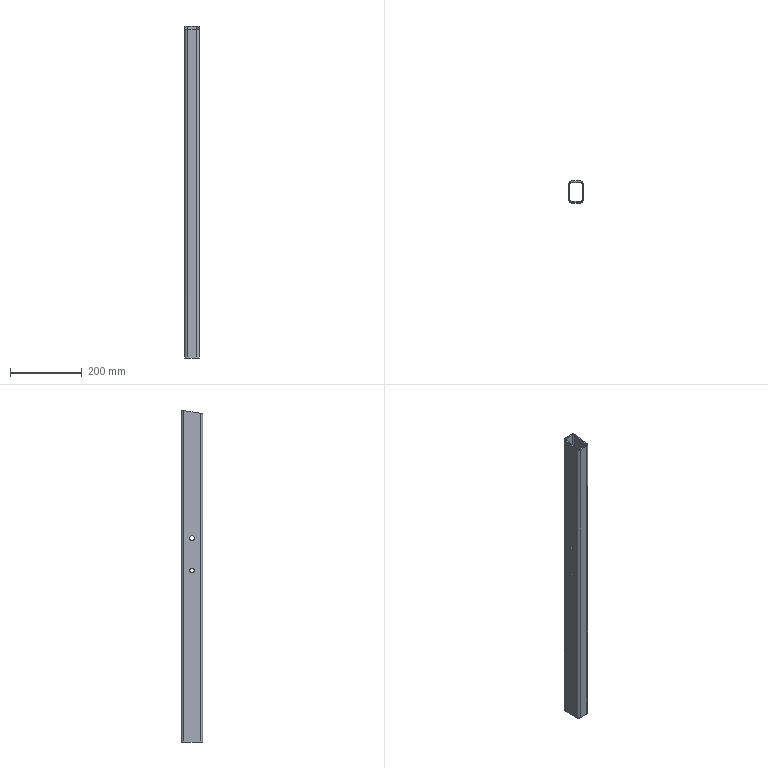Part | SolidWorks | features BaseBody 1 | 1 solid | 26 faces | box 40 x 60 x 928.577 mm | volume 490609 mm3 | cylinder 16 | plane 10 | commonest cylinder face diameters 13 x8 9 x4 15 x4
STEP:
#1=CARTESIAN_POINT('',(-20.,0.,576.5));
#2=VERTEX_POINT('',#1);
#3=CARTESIAN_POINT('',(-20.,0.,563.5));
#4=VERTEX_POINT('',#3);
#5=CARTESIAN_POINT('',(-20.,0.,570.));
#6=DIRECTION('',(1.,0.,0.));
#7=DIRECTION('',(0.,0.,-1.));
#8=AXIS2_PLACEMENT_3D('',#5,#6,#7);
#9=CIRCLE('',#8,6.5);
#10=EDGE_CURVE('',#2,#4,#9,.T.);
#11=ORIENTED_EDGE('',*,*,#10,.F.);
#12=CARTESIAN_POINT('',(-17.,0.,576.5));
#13=VERTEX_POINT('',#12);
#14=CARTESIAN_POINT('',(-911.372,0.,576.5));
#15=DIRECTION('',(1.,0.,0.));
#16=VECTOR('',#15,1000.);
#17=LINE('',#14,#16);
#18=EDGE_CURVE('',#2,#13,#17,.T.);
#19=ORIENTED_EDGE('',*,*,#18,.T.);
#20=CARTESIAN_POINT('',(-17.,0.,563.5));
#21=VERTEX_POINT('',#20);
#22=CARTESIAN_POINT('',(-17.,0.,570.));
#23=DIRECTION('',(1.,0.,0.));
#24=DIRECTION('',(0.,0.,-1.));
#25=AXIS2_PLACEMENT_3D('',#22,#23,#24);
#26=CIRCLE('',#25,6.5);
#27=EDGE_CURVE('',#13,#21,#26,.T.);
#28=ORIENTED_EDGE('',*,*,#27,.T.);
#29=CARTESIAN_POINT('',(-911.372,0.,563.5));
#30=DIRECTION('',(1.,0.,0.));
#31=VECTOR('',#30,1000.);
#32=LINE('',#29,#31);
#33=EDGE_CURVE('',#4,#21,#32,.T.);
#34=ORIENTED_EDGE('',*,*,#33,.F.);
#35=EDGE_LOOP('',(#11,#19,#28,#34));
#36=FACE_OUTER_BOUND('',#35,.T.);
#37=CARTESIAN_POINT('',(-911.372,0.,570.));
#38=DIRECTION('',(1.,0.,0.));
#39=DIRECTION('',(0.,0.,-1.));
#40=AXIS2_PLACEMENT_3D('',#37,#38,#39);
#41=CYLINDRICAL_SURFACE('',#40,6.5);
#42=ADVANCED_FACE('',(#36),#41,.F.);
#43=CARTESIAN_POINT('',(-20.,0.,486.5));
#44=VERTEX_POINT('',#43);
#45=CARTESIAN_POINT('',(-20.,0.,473.5));
#46=VERTEX_POINT('',#45);
#47=CARTESIAN_POINT('',(-20.,0.,480.));
#48=DIRECTION('',(1.,0.,0.));
#49=DIRECTION('',(0.,0.,-1.));
#50=AXIS2_PLACEMENT_3D('',#47,#48,#49);
#51=CIRCLE('',#50,6.5);
#52=EDGE_CURVE('',#44,#46,#51,.T.);
#53=ORIENTED_EDGE('',*,*,#52,.F.);
#54=CARTESIAN_POINT('',(-17.,0.,486.5));
#55=VERTEX_POINT('',#54);
#56=CARTESIAN_POINT('',(-911.372,0.,486.5));
#57=DIRECTION('',(1.,0.,0.));
#58=VECTOR('',#57,1000.);
#59=LINE('',#56,#58);
#60=EDGE_CURVE('',#44,#55,#59,.T.);
#61=ORIENTED_EDGE('',*,*,#60,.T.);
#62=CARTESIAN_POINT('',(-17.,0.,473.5));
#63=VERTEX_POINT('',#62);
#64=CARTESIAN_POINT('',(-17.,0.,480.));
#65=DIRECTION('',(1.,0.,0.));
#66=DIRECTION('',(0.,0.,-1.));
#67=AXIS2_PLACEMENT_3D('',#64,#65,#66);
#68=CIRCLE('',#67,6.5);
#69=EDGE_CURVE('',#55,#63,#68,.T.);
#70=ORIENTED_EDGE('',*,*,#69,.T.);
#71=CARTESIAN_POINT('',(-911.372,0.,473.5));
#72=DIRECTION('',(1.,0.,0.));
#73=VECTOR('',#72,1000.);
#74=LINE('',#71,#73);
#75=EDGE_CURVE('',#46,#63,#74,.T.);
#76=ORIENTED_EDGE('',*,*,#75,.F.);
#77=EDGE_LOOP('',(#53,#61,#70,#76));
#78=FACE_OUTER_BOUND('',#77,.T.);
#79=CARTESIAN_POINT('',(-911.372,0.,480.));
#80=DIRECTION('',(1.,0.,0.));
#81=DIRECTION('',(0.,0.,-1.));
#82=AXIS2_PLACEMENT_3D('',#79,#80,#81);
#83=CYLINDRICAL_SURFACE('',#82,6.5);
#84=ADVANCED_FACE('',(#78),#83,.F.);
#85=CARTESIAN_POINT('',(17.,0.,563.5));
#86=VERTEX_POINT('',#85);
#87=CARTESIAN_POINT('',(17.,0.,576.5));
#88=VERTEX_POINT('',#87);
#89=CARTESIAN_POINT('',(17.,0.,570.));
#90=DIRECTION('',(-1.,0.,0.));
#91=DIRECTION('',(0.,0.,-1.));
#92=AXIS2_PLACEMENT_3D('',#89,#90,#91);
#93=CIRCLE('',#92,6.5);
#94=EDGE_CURVE('',#86,#88,#93,.T.);
#95=ORIENTED_EDGE('',*,*,#94,.T.);
#96=CARTESIAN_POINT('',(20.,0.,576.5));
#97=VERTEX_POINT('',#96);
#98=CARTESIAN_POINT('',(-911.372,0.,576.5));
#99=DIRECTION('',(1.,0.,0.));
#100=VECTOR('',#99,1000.);
#101=LINE('',#98,#100);
#102=EDGE_CURVE('',#88,#97,#101,.T.);
#103=ORIENTED_EDGE('',*,*,#102,.T.);
#104=CARTESIAN_POINT('',(20.,0.,563.5));
#105=VERTEX_POINT('',#104);
#106=CARTESIAN_POINT('',(20.,0.,570.));
#107=DIRECTION('',(-1.,0.,0.));
#108=DIRECTION('',(0.,0.,-1.));
#109=AXIS2_PLACEMENT_3D('',#106,#107,#108);
#110=CIRCLE('',#109,6.5);
#111=EDGE_CURVE('',#105,#97,#110,.T.);
#112=ORIENTED_EDGE('',*,*,#111,.F.);
#113=CARTESIAN_POINT('',(-911.372,0.,563.5));
#114=DIRECTION('',(1.,0.,0.));
#115=VECTOR('',#114,1000.);
#116=LINE('',#113,#115);
#117=EDGE_CURVE('',#86,#105,#116,.T.);
#118=ORIENTED_EDGE('',*,*,#117,.F.);
#119=EDGE_LOOP('',(#95,#103,#112,#118));
#120=FACE_OUTER_BOUND('',#119,.T.);
#121=CARTESIAN_POINT('',(-911.372,0.,570.));
#122=DIRECTION('',(1.,0.,0.));
#123=DIRECTION('',(0.,0.,-1.));
#124=AXIS2_PLACEMENT_3D('',#121,#122,#123);
#125=CYLINDRICAL_SURFACE('',#124,6.5);
#126=ADVANCED_FACE('',(#120),#125,.F.);
#127=CARTESIAN_POINT('',(17.,0.,473.5));
#128=VERTEX_POINT('',#127);
#129=CARTESIAN_POINT('',(17.,0.,486.5));
#130=VERTEX_POINT('',#129);
#131=CARTESIAN_POINT('',(17.,0.,480.));
#132=DIRECTION('',(-1.,0.,0.));
#133=DIRECTION('',(0.,0.,-1.));
#134=AXIS2_PLACEMENT_3D('',#131,#132,#133);
#135=CIRCLE('',#134,6.5);
#136=EDGE_CURVE('',#128,#130,#135,.T.);
#137=ORIENTED_EDGE('',*,*,#136,.T.);
#138=CARTESIAN_POINT('',(20.,0.,486.5));
#139=VERTEX_POINT('',#138);
#140=CARTESIAN_POINT('',(-911.372,0.,486.5));
#141=DIRECTION('',(1.,0.,0.));
#142=VECTOR('',#141,1000.);
#143=LINE('',#140,#142);
#144=EDGE_CURVE('',#130,#139,#143,.T.);
#145=ORIENTED_EDGE('',*,*,#144,.T.);
#146=CARTESIAN_POINT('',(20.,0.,473.5));
#147=VERTEX_POINT('',#146);
#148=CARTESIAN_POINT('',(20.,0.,480.));
#149=DIRECTION('',(-1.,0.,0.));
#150=DIRECTION('',(0.,0.,-1.));
#151=AXIS2_PLACEMENT_3D('',#148,#149,#150);
#152=CIRCLE('',#151,6.5);
#153=EDGE_CURVE('',#147,#139,#152,.T.);
#154=ORIENTED_EDGE('',*,*,#153,.F.);
#155=CARTESIAN_POINT('',(-911.372,0.,473.5));
#156=DIRECTION('',(1.,0.,0.));
#157=VECTOR('',#156,1000.);
#158=LINE('',#155,#157);
#159=EDGE_CURVE('',#128,#147,#158,.T.);
#160=ORIENTED_EDGE('',*,*,#159,.F.);
#161=EDGE_LOOP('',(#137,#145,#154,#160));
#162=FACE_OUTER_BOUND('',#161,.T.);
#163=CARTESIAN_POINT('',(-911.372,0.,480.));
#164=DIRECTION('',(1.,0.,0.));
#165=DIRECTION('',(0.,0.,-1.));
#166=AXIS2_PLACEMENT_3D('',#163,#164,#165);
#167=CYLINDRICAL_SURFACE('',#166,6.5);
#168=ADVANCED_FACE('',(#162),#167,.F.);
#169=CARTESIAN_POINT('',(-17.,0.,570.));
#170=DIRECTION('',(1.,0.,0.));
#171=DIRECTION('',(0.,0.,-1.));
#172=AXIS2_PLACEMENT_3D('',#169,#170,#171);
#173=CIRCLE('',#172,6.5);
#174=EDGE_CURVE('',#21,#13,#173,.T.);
#175=ORIENTED_EDGE('',*,*,#174,.F.);
#176=ORIENTED_EDGE('',*,*,#27,.F.);
#177=EDGE_LOOP('',(#175,#176));
#178=FACE_BOUND('',#177,.T.);
#179=CARTESIAN_POINT('',(-17.,0.,480.));
#180=DIRECTION('',(1.,0.,0.));
#181=DIRECTION('',(0.,0.,-1.));
#182=AXIS2_PLACEMENT_3D('',#179,#180,#181);
#183=CIRCLE('',#182,6.5);
#184=EDGE_CURVE('',#63,#55,#183,.T.);
#185=ORIENTED_EDGE('',*,*,#184,.F.);
#186=ORIENTED_EDGE('',*,*,#69,.F.);
#187=EDGE_LOOP('',(#185,#186));
#188=FACE_BOUND('',#187,.T.);
#189=CARTESIAN_POINT('',(-17.,-22.5,0.));
#190=VERTEX_POINT('',#189);
#191=CARTESIAN_POINT('',(-17.,-22.5,919.319));
#192=VERTEX_POINT('',#191);
#193=CARTESIAN_POINT('',(-17.,-22.5,0.));
#194=DIRECTION('',(0.,0.,1.));
#195=VECTOR('',#194,1000.);
#196=LINE('',#193,#195);
#197=EDGE_CURVE('',#190,#192,#196,.T.);
#198=ORIENTED_EDGE('',*,*,#197,.F.);
#199=CARTESIAN_POINT('',(-17.,22.5,0.));
#200=VERTEX_POINT('',#199);
#201=CARTESIAN_POINT('',(-17.,-22.5,0.));
#202=DIRECTION('',(0.,-1.,0.));
#203=VECTOR('',#202,1000.);
#204=LINE('',#201,#203);
#205=EDGE_CURVE('',#200,#190,#204,.T.);
#206=ORIENTED_EDGE('',*,*,#205,.F.);
#207=CARTESIAN_POINT('',(-17.,22.5,927.254));
#208=VERTEX_POINT('',#207);
#209=CARTESIAN_POINT('',(-17.,22.5,0.));
#210=DIRECTION('',(0.,0.,-1.));
#211=VECTOR('',#210,1000.);
#212=LINE('',#209,#211);
#213=EDGE_CURVE('',#208,#200,#212,.T.);
#214=ORIENTED_EDGE('',*,*,#213,.F.);
#215=CARTESIAN_POINT('',(-17.,-22.5,919.319));
#216=DIRECTION('',(0.,0.9848,0.1736));
#217=VECTOR('',#216,1000.);
#218=LINE('',#215,#217);
#219=EDGE_CURVE('',#192,#208,#218,.T.);
#220=ORIENTED_EDGE('',*,*,#219,.F.);
#221=EDGE_LOOP('',(#198,#206,#214,#220));
#222=FACE_OUTER_BOUND('',#221,.T.);
#223=CARTESIAN_POINT('',(-17.,-22.5,0.));
#224=DIRECTION('',(-1.,0.,0.));
#225=DIRECTION('',(0.,-1.,0.));
#226=AXIS2_PLACEMENT_3D('',#223,#224,#225);
#227=PLANE('',#226);
#228=ADVANCED_FACE('',(#178,#188,#222),#227,.F.);
#229=ORIENTED_EDGE('',*,*,#18,.F.);
#230=CARTESIAN_POINT('',(-20.,0.,570.));
#231=DIRECTION('',(1.,0.,0.));
#232=DIRECTION('',(0.,0.,-1.));
#233=AXIS2_PLACEMENT_3D('',#230,#231,#232);
#234=CIRCLE('',#233,6.5);
#235=EDGE_CURVE('',#4,#2,#234,.T.);
#236=ORIENTED_EDGE('',*,*,#235,.F.);
#237=ORIENTED_EDGE('',*,*,#33,.T.);
#238=ORIENTED_EDGE('',*,*,#174,.T.);
#239=EDGE_LOOP('',(#229,#236,#237,#238));
#240=FACE_OUTER_BOUND('',#239,.T.);
#241=CARTESIAN_POINT('',(-911.372,0.,570.));
#242=DIRECTION('',(1.,0.,0.));
#243=DIRECTION('',(0.,0.,-1.));
#244=AXIS2_PLACEMENT_3D('',#241,#242,#243);
#245=CYLINDRICAL_SURFACE('',#244,6.5);
#246=ADVANCED_FACE('',(#240),#245,.F.);
#247=ORIENTED_EDGE('',*,*,#60,.F.);
#248=CARTESIAN_POINT('',(-20.,0.,480.));
#249=DIRECTION('',(1.,0.,0.));
#250=DIRECTION('',(0.,0.,-1.));
#251=AXIS2_PLACEMENT_3D('',#248,#249,#250);
#252=CIRCLE('',#251,6.5);
#253=EDGE_CURVE('',#46,#44,#252,.T.);
#254=ORIENTED_EDGE('',*,*,#253,.F.);
#255=ORIENTED_EDGE('',*,*,#75,.T.);
#256=ORIENTED_EDGE('',*,*,#184,.T.);
#257=EDGE_LOOP('',(#247,#254,#255,#256));
#258=FACE_OUTER_BOUND('',#257,.T.);
#259=CARTESIAN_POINT('',(-911.372,0.,480.));
#260=DIRECTION('',(1.,0.,0.));
#261=DIRECTION('',(0.,0.,-1.));
#262=AXIS2_PLACEMENT_3D('',#259,#260,#261);
#263=CYLINDRICAL_SURFACE('',#262,6.5);
#264=ADVANCED_FACE('',(#258),#263,.F.);
#265=CARTESIAN_POINT('',(-12.5,-27.,918.526));
#266=VERTEX_POINT('',#265);
#267=CARTESIAN_POINT('',(-17.,-22.5,919.319));
#268=CARTESIAN_POINT('',(-17.,-25.136,918.855));
#269=CARTESIAN_POINT('',(-15.136,-27.,918.526));
#270=CARTESIAN_POINT('',(-12.5,-27.,918.526));
#271=(BOUNDED_CURVE()B_SPLINE_CURVE(3,(#267,#268,#269,#270),.UNSPECIFIED.,.F.,.F.)B_SPLINE_CURVE_WITH_KNOTS((4,4),(1.571,3.142),.UNSPECIFIED.)CURVE()GEOMETRIC_REPRESENTATION_ITEM()RATIONAL_B_SPLINE_CURVE((1.,0.8047,0.8047,1.))REPRESENTATION_ITEM(''));
#272=EDGE_CURVE('',#192,#266,#271,.T.);
#273=ORIENTED_EDGE('',*,*,#272,.F.);
#274=ORIENTED_EDGE('',*,*,#219,.T.);
#275=CARTESIAN_POINT('',(-12.5,27.,928.048));
#276=VERTEX_POINT('',#275);
#277=CARTESIAN_POINT('',(-12.5,27.,928.048));
#278=CARTESIAN_POINT('',(-15.136,27.,928.048));
#279=CARTESIAN_POINT('',(-17.,25.136,927.719));
#280=CARTESIAN_POINT('',(-17.,22.5,927.254));
#281=(BOUNDED_CURVE()B_SPLINE_CURVE(3,(#277,#278,#279,#280),.UNSPECIFIED.,.F.,.F.)B_SPLINE_CURVE_WITH_KNOTS((4,4),(0.,1.571),.UNSPECIFIED.)CURVE()GEOMETRIC_REPRESENTATION_ITEM()RATIONAL_B_SPLINE_CURVE((1.,0.8047,0.8047,1.))REPRESENTATION_ITEM(''));
#282=EDGE_CURVE('',#276,#208,#281,.T.);
#283=ORIENTED_EDGE('',*,*,#282,.F.);
#284=CARTESIAN_POINT('',(12.5,27.,928.048));
#285=VERTEX_POINT('',#284);
#286=CARTESIAN_POINT('',(0.,27.,928.048));
#287=DIRECTION('',(-1.,0.,0.));
#288=VECTOR('',#287,1000.);
#289=LINE('',#286,#288);
#290=EDGE_CURVE('',#285,#276,#289,.T.);
#291=ORIENTED_EDGE('',*,*,#290,.F.);
#292=CARTESIAN_POINT('',(17.,22.5,927.254));
#293=VERTEX_POINT('',#292);
#294=CARTESIAN_POINT('',(17.,22.5,927.254));
#295=CARTESIAN_POINT('',(17.,25.136,927.719));
#296=CARTESIAN_POINT('',(15.136,27.,928.048));
#297=CARTESIAN_POINT('',(12.5,27.,928.048));
#298=(BOUNDED_CURVE()B_SPLINE_CURVE(3,(#294,#295,#296,#297),.UNSPECIFIED.,.F.,.F.)B_SPLINE_CURVE_WITH_KNOTS((4,4),(4.712,6.283),.UNSPECIFIED.)CURVE()GEOMETRIC_REPRESENTATION_ITEM()RATIONAL_B_SPLINE_CURVE((1.,0.8047,0.8047,1.))REPRESENTATION_ITEM(''));
#299=EDGE_CURVE('',#293,#285,#298,.T.);
#300=ORIENTED_EDGE('',*,*,#299,.F.);
#301=CARTESIAN_POINT('',(17.,-22.5,919.319));
#302=VERTEX_POINT('',#301);
#303=CARTESIAN_POINT('',(17.,-157.891,895.446));
#304=DIRECTION('',(0.,0.9848,0.1736));
#305=VECTOR('',#304,1000.);
#306=LINE('',#303,#305);
#307=EDGE_CURVE('',#302,#293,#306,.T.);
#308=ORIENTED_EDGE('',*,*,#307,.F.);
#309=CARTESIAN_POINT('',(12.5,-27.,918.526));
#310=VERTEX_POINT('',#309);
#311=CARTESIAN_POINT('',(12.5,-27.,918.526));
#312=CARTESIAN_POINT('',(15.136,-27.,918.526));
#313=CARTESIAN_POINT('',(17.,-25.136,918.855));
#314=CARTESIAN_POINT('',(17.,-22.5,919.319));
#315=(BOUNDED_CURVE()B_SPLINE_CURVE(3,(#311,#312,#313,#314),.UNSPECIFIED.,.F.,.T.)B_SPLINE_CURVE_WITH_KNOTS((4,4),(3.142,4.712),.UNSPECIFIED.)CURVE()GEOMETRIC_REPRESENTATION_ITEM()RATIONAL_B_SPLINE_CURVE((1.,0.8047,0.8047,1.))REPRESENTATION_ITEM(''));
#316=EDGE_CURVE('',#310,#302,#315,.T.);
#317=ORIENTED_EDGE('',*,*,#316,.F.);
#318=CARTESIAN_POINT('',(0.,-27.,918.526));
#319=DIRECTION('',(1.,0.,0.));
#320=VECTOR('',#319,1000.);
#321=LINE('',#318,#320);
#322=EDGE_CURVE('',#266,#310,#321,.T.);
#323=ORIENTED_EDGE('',*,*,#322,.F.);
#324=EDGE_LOOP('',(#273,#274,#283,#291,#300,#308,#317,#323));
#325=FACE_BOUND('',#324,.T.);
#326=CARTESIAN_POINT('',(12.5,30.,928.577));
#327=VERTEX_POINT('',#326);
#328=CARTESIAN_POINT('',(20.,22.5,927.254));
#329=VERTEX_POINT('',#328);
#330=CARTESIAN_POINT('',(12.5,30.,928.577));
#331=CARTESIAN_POINT('',(16.893,30.,928.577));
#332=CARTESIAN_POINT('',(20.,26.893,928.029));
#333=CARTESIAN_POINT('',(20.,22.5,927.254));
#334=(BOUNDED_CURVE()B_SPLINE_CURVE(3,(#330,#331,#332,#333),.UNSPECIFIED.,.F.,.F.)B_SPLINE_CURVE_WITH_KNOTS((4,4),(0.,1.571),.UNSPECIFIED.)CURVE()GEOMETRIC_REPRESENTATION_ITEM()RATIONAL_B_SPLINE_CURVE((1.,0.8047,0.8047,1.))REPRESENTATION_ITEM(''));
#335=EDGE_CURVE('',#327,#329,#334,.T.);
#336=ORIENTED_EDGE('',*,*,#335,.F.);
#337=CARTESIAN_POINT('',(-12.5,30.,928.577));
#338=VERTEX_POINT('',#337);
#339=CARTESIAN_POINT('',(0.,30.,928.577));
#340=DIRECTION('',(1.,0.,0.));
#341=VECTOR('',#340,1000.);
#342=LINE('',#339,#341);
#343=EDGE_CURVE('',#338,#327,#342,.T.);
#344=ORIENTED_EDGE('',*,*,#343,.F.);
#345=CARTESIAN_POINT('',(-20.,22.5,927.254));
#346=VERTEX_POINT('',#345);
#347=CARTESIAN_POINT('',(-20.,22.5,927.254));
#348=CARTESIAN_POINT('',(-20.,26.893,928.029));
#349=CARTESIAN_POINT('',(-16.893,30.,928.577));
#350=CARTESIAN_POINT('',(-12.5,30.,928.577));
#351=(BOUNDED_CURVE()B_SPLINE_CURVE(3,(#347,#348,#349,#350),.UNSPECIFIED.,.F.,.F.)B_SPLINE_CURVE_WITH_KNOTS((4,4),(4.712,6.283),.UNSPECIFIED.)CURVE()GEOMETRIC_REPRESENTATION_ITEM()RATIONAL_B_SPLINE_CURVE((1.,0.8047,0.8047,1.))REPRESENTATION_ITEM(''));
#352=EDGE_CURVE('',#346,#338,#351,.T.);
#353=ORIENTED_EDGE('',*,*,#352,.F.);
#354=CARTESIAN_POINT('',(-20.,-22.5,919.319));
#355=VERTEX_POINT('',#354);
#356=CARTESIAN_POINT('',(-20.,-157.891,895.446));
#357=DIRECTION('',(0.,0.9848,0.1736));
#358=VECTOR('',#357,1000.);
#359=LINE('',#356,#358);
#360=EDGE_CURVE('',#355,#346,#359,.T.);
#361=ORIENTED_EDGE('',*,*,#360,.F.);
#362=CARTESIAN_POINT('',(-12.5,-30.,917.997));
#363=VERTEX_POINT('',#362);
#364=CARTESIAN_POINT('',(-12.5,-30.,917.997));
#365=CARTESIAN_POINT('',(-16.893,-30.,917.997));
#366=CARTESIAN_POINT('',(-20.,-26.893,918.545));
#367=CARTESIAN_POINT('',(-20.,-22.5,919.319));
#368=(BOUNDED_CURVE()B_SPLINE_CURVE(3,(#364,#365,#366,#367),.UNSPECIFIED.,.F.,.F.)B_SPLINE_CURVE_WITH_KNOTS((4,4),(3.142,4.712),.UNSPECIFIED.)CURVE()GEOMETRIC_REPRESENTATION_ITEM()RATIONAL_B_SPLINE_CURVE((1.,0.8047,0.8047,1.))REPRESENTATION_ITEM(''));
#369=EDGE_CURVE('',#363,#355,#368,.T.);
#370=ORIENTED_EDGE('',*,*,#369,.F.);
#371=CARTESIAN_POINT('',(12.5,-30.,917.997));
#372=VERTEX_POINT('',#371);
#373=CARTESIAN_POINT('',(0.,-30.,917.997));
#374=DIRECTION('',(-1.,0.,0.));
#375=VECTOR('',#374,1000.);
#376=LINE('',#373,#375);
#377=EDGE_CURVE('',#372,#363,#376,.T.);
#378=ORIENTED_EDGE('',*,*,#377,.F.);
#379=CARTESIAN_POINT('',(20.,-22.5,919.319));
#380=VERTEX_POINT('',#379);
#381=CARTESIAN_POINT('',(20.,-22.5,919.319));
#382=CARTESIAN_POINT('',(20.,-26.893,918.545));
#383=CARTESIAN_POINT('',(16.893,-30.,917.997));
#384=CARTESIAN_POINT('',(12.5,-30.,917.997));
#385=(BOUNDED_CURVE()B_SPLINE_CURVE(3,(#381,#382,#383,#384),.UNSPECIFIED.,.F.,.F.)B_SPLINE_CURVE_WITH_KNOTS((4,4),(1.571,3.142),.UNSPECIFIED.)CURVE()GEOMETRIC_REPRESENTATION_ITEM()RATIONAL_B_SPLINE_CURVE((1.,0.8047,0.8047,1.))REPRESENTATION_ITEM(''));
#386=EDGE_CURVE('',#380,#372,#385,.T.);
#387=ORIENTED_EDGE('',*,*,#386,.F.);
#388=CARTESIAN_POINT('',(20.,-157.891,895.446));
#389=DIRECTION('',(0.,-0.9848,-0.1736));
#390=VECTOR('',#389,1000.);
#391=LINE('',#388,#390);
#392=EDGE_CURVE('',#329,#380,#391,.T.);
#393=ORIENTED_EDGE('',*,*,#392,.F.);
#394=EDGE_LOOP('',(#336,#344,#353,#361,#370,#378,#387,#393));
#395=FACE_OUTER_BOUND('',#394,.T.);
#396=CARTESIAN_POINT('',(0.,-157.891,895.446));
#397=DIRECTION('',(0.,0.1736,-0.9848));
#398=DIRECTION('',(0.,0.9848,0.1736));
#399=AXIS2_PLACEMENT_3D('',#396,#397,#398);
#400=PLANE('',#399);
#401=ADVANCED_FACE('',(#325,#395),#400,.F.);
#402=CARTESIAN_POINT('',(-12.5,-27.,0.));
#403=VERTEX_POINT('',#402);
#404=CARTESIAN_POINT('',(-12.5,-27.,0.));
#405=DIRECTION('',(0.,0.,1.));
#406=VECTOR('',#405,1000.);
#407=LINE('',#404,#406);
#408=EDGE_CURVE('',#403,#266,#407,.T.);
#409=ORIENTED_EDGE('',*,*,#408,.F.);
#410=CARTESIAN_POINT('',(-12.5,-22.5,0.));
#411=DIRECTION('',(0.,0.,1.));
#412=DIRECTION('',(1.,0.,0.));
#413=AXIS2_PLACEMENT_3D('',#410,#411,#412);
#414=CIRCLE('',#413,4.5);
#415=EDGE_CURVE('',#190,#403,#414,.T.);
#416=ORIENTED_EDGE('',*,*,#415,.F.);
#417=ORIENTED_EDGE('',*,*,#197,.T.);
#418=ORIENTED_EDGE('',*,*,#272,.T.);
#419=EDGE_LOOP('',(#409,#416,#417,#418));
#420=FACE_OUTER_BOUND('',#419,.T.);
#421=CARTESIAN_POINT('',(-12.5,-22.5,0.));
#422=DIRECTION('',(0.,0.,1.));
#423=DIRECTION('',(1.,0.,0.));
#424=AXIS2_PLACEMENT_3D('',#421,#422,#423);
#425=CYLINDRICAL_SURFACE('',#424,4.5);
#426=ADVANCED_FACE('',(#420),#425,.F.);
#427=CARTESIAN_POINT('',(-12.5,27.,0.));
#428=VERTEX_POINT('',#427);
#429=CARTESIAN_POINT('',(-12.5,22.5,0.));
#430=DIRECTION('',(0.,0.,-1.));
#431=DIRECTION('',(1.,0.,0.));
#432=AXIS2_PLACEMENT_3D('',#429,#430,#431);
#433=CIRCLE('',#432,4.5);
#434=EDGE_CURVE('',#200,#428,#433,.T.);
#435=ORIENTED_EDGE('',*,*,#434,.F.);
#436=ORIENTED_EDGE('',*,*,#205,.T.);
#437=ORIENTED_EDGE('',*,*,#415,.T.);
#438=CARTESIAN_POINT('',(12.5,-27.,0.));
#439=VERTEX_POINT('',#438);
#440=CARTESIAN_POINT('',(0.,-27.,0.));
#441=DIRECTION('',(-1.,0.,0.));
#442=VECTOR('',#441,1000.);
#443=LINE('',#440,#442);
#444=EDGE_CURVE('',#439,#403,#443,.T.);
#445=ORIENTED_EDGE('',*,*,#444,.F.);
#446=CARTESIAN_POINT('',(17.,-22.5,0.));
#447=VERTEX_POINT('',#446);
#448=CARTESIAN_POINT('',(12.5,-22.5,0.));
#449=DIRECTION('',(0.,0.,-1.));
#450=DIRECTION('',(1.,0.,0.));
#451=AXIS2_PLACEMENT_3D('',#448,#449,#450);
#452=CIRCLE('',#451,4.5);
#453=EDGE_CURVE('',#447,#439,#452,.T.);
#454=ORIENTED_EDGE('',*,*,#453,.F.);
#455=CARTESIAN_POINT('',(17.,22.5,0.));
#456=VERTEX_POINT('',#455);
#457=CARTESIAN_POINT('',(17.,0.,0.));
#458=DIRECTION('',(0.,-1.,0.));
#459=VECTOR('',#458,1000.);
#460=LINE('',#457,#459);
#461=EDGE_CURVE('',#456,#447,#460,.T.);
#462=ORIENTED_EDGE('',*,*,#461,.F.);
#463=CARTESIAN_POINT('',(12.5,27.,0.));
#464=VERTEX_POINT('',#463);
#465=CARTESIAN_POINT('',(12.5,22.5,0.));
#466=DIRECTION('',(0.,0.,-1.));
#467=DIRECTION('',(1.,0.,0.));
#468=AXIS2_PLACEMENT_3D('',#465,#466,#467);
#469=CIRCLE('',#468,4.5);
#470=EDGE_CURVE('',#464,#456,#469,.T.);
#471=ORIENTED_EDGE('',*,*,#470,.F.);
#472=CARTESIAN_POINT('',(0.,27.,0.));
#473=DIRECTION('',(1.,0.,0.));
#474=VECTOR('',#473,1000.);
#475=LINE('',#472,#474);
#476=EDGE_CURVE('',#428,#464,#475,.T.);
#477=ORIENTED_EDGE('',*,*,#476,.F.);
#478=EDGE_LOOP('',(#435,#436,#437,#445,#454,#462,#471,#477));
#479=FACE_BOUND('',#478,.T.);
#480=CARTESIAN_POINT('',(-12.5,30.,0.));
#481=VERTEX_POINT('',#480);
#482=CARTESIAN_POINT('',(-20.,22.5,0.));
#483=VERTEX_POINT('',#482);
#484=CARTESIAN_POINT('',(-12.5,22.5,0.));
#485=DIRECTION('',(0.,0.,1.));
#486=DIRECTION('',(1.,0.,0.));
#487=AXIS2_PLACEMENT_3D('',#484,#485,#486);
#488=CIRCLE('',#487,7.5);
#489=EDGE_CURVE('',#481,#483,#488,.T.);
#490=ORIENTED_EDGE('',*,*,#489,.F.);
#491=CARTESIAN_POINT('',(12.5,30.,0.));
#492=VERTEX_POINT('',#491);
#493=CARTESIAN_POINT('',(0.,30.,0.));
#494=DIRECTION('',(-1.,0.,0.));
#495=VECTOR('',#494,1000.);
#496=LINE('',#493,#495);
#497=EDGE_CURVE('',#492,#481,#496,.T.);
#498=ORIENTED_EDGE('',*,*,#497,.F.);
#499=CARTESIAN_POINT('',(20.,22.5,0.));
#500=VERTEX_POINT('',#499);
#501=CARTESIAN_POINT('',(12.5,22.5,0.));
#502=DIRECTION('',(0.,0.,1.));
#503=DIRECTION('',(1.,0.,0.));
#504=AXIS2_PLACEMENT_3D('',#501,#502,#503);
#505=CIRCLE('',#504,7.5);
#506=EDGE_CURVE('',#500,#492,#505,.T.);
#507=ORIENTED_EDGE('',*,*,#506,.F.);
#508=CARTESIAN_POINT('',(20.,-22.5,0.));
#509=VERTEX_POINT('',#508);
#510=CARTESIAN_POINT('',(20.,0.,0.));
#511=DIRECTION('',(0.,1.,0.));
#512=VECTOR('',#511,1000.);
#513=LINE('',#510,#512);
#514=EDGE_CURVE('',#509,#500,#513,.T.);
#515=ORIENTED_EDGE('',*,*,#514,.F.);
#516=CARTESIAN_POINT('',(12.5,-30.,0.));
#517=VERTEX_POINT('',#516);
#518=CARTESIAN_POINT('',(12.5,-22.5,0.));
#519=DIRECTION('',(0.,0.,1.));
#520=DIRECTION('',(1.,0.,0.));
#521=AXIS2_PLACEMENT_3D('',#518,#519,#520);
#522=CIRCLE('',#521,7.5);
#523=EDGE_CURVE('',#517,#509,#522,.T.);
#524=ORIENTED_EDGE('',*,*,#523,.F.);
#525=CARTESIAN_POINT('',(-12.5,-30.,0.));
#526=VERTEX_POINT('',#525);
#527=CARTESIAN_POINT('',(0.,-30.,0.));
#528=DIRECTION('',(1.,0.,0.));
#529=VECTOR('',#528,1000.);
#530=LINE('',#527,#529);
#531=EDGE_CURVE('',#526,#517,#530,.T.);
#532=ORIENTED_EDGE('',*,*,#531,.F.);
#533=CARTESIAN_POINT('',(-20.,-22.5,0.));
#534=VERTEX_POINT('',#533);
#535=CARTESIAN_POINT('',(-12.5,-22.5,0.));
#536=DIRECTION('',(0.,0.,1.));
#537=DIRECTION('',(1.,0.,0.));
#538=AXIS2_PLACEMENT_3D('',#535,#536,#537);
#539=CIRCLE('',#538,7.5);
#540=EDGE_CURVE('',#534,#526,#539,.T.);
#541=ORIENTED_EDGE('',*,*,#540,.F.);
#542=CARTESIAN_POINT('',(-20.,0.,0.));
#543=DIRECTION('',(0.,-1.,0.));
#544=VECTOR('',#543,1000.);
#545=LINE('',#542,#544);
#546=EDGE_CURVE('',#483,#534,#545,.T.);
#547=ORIENTED_EDGE('',*,*,#546,.F.);
#548=EDGE_LOOP('',(#490,#498,#507,#515,#524,#532,#541,#547));
#549=FACE_OUTER_BOUND('',#548,.T.);
#550=CARTESIAN_POINT('',(0.,0.,0.));
#551=DIRECTION('',(0.,0.,1.));
#552=DIRECTION('',(1.,0.,0.));
#553=AXIS2_PLACEMENT_3D('',#550,#551,#552);
#554=PLANE('',#553);
#555=ADVANCED_FACE('',(#479,#549),#554,.F.);
#556=ORIENTED_EDGE('',*,*,#213,.T.);
#557=ORIENTED_EDGE('',*,*,#434,.T.);
#558=CARTESIAN_POINT('',(-12.5,27.,0.));
#559=DIRECTION('',(0.,0.,-1.));
#560=VECTOR('',#559,1000.);
#561=LINE('',#558,#560);
#562=EDGE_CURVE('',#276,#428,#561,.T.);
#563=ORIENTED_EDGE('',*,*,#562,.F.);
#564=ORIENTED_EDGE('',*,*,#282,.T.);
#565=EDGE_LOOP('',(#556,#557,#563,#564));
#566=FACE_OUTER_BOUND('',#565,.T.);
#567=CARTESIAN_POINT('',(-12.5,22.5,0.));
#568=DIRECTION('',(0.,0.,1.));
#569=DIRECTION('',(1.,0.,0.));
#570=AXIS2_PLACEMENT_3D('',#567,#568,#569);
#571=CYLINDRICAL_SURFACE('',#570,4.5);
#572=ADVANCED_FACE('',(#566),#571,.F.);
#573=ORIENTED_EDGE('',*,*,#235,.T.);
#574=ORIENTED_EDGE('',*,*,#10,.T.);
#575=EDGE_LOOP('',(#573,#574));
#576=FACE_BOUND('',#575,.T.);
#577=ORIENTED_EDGE('',*,*,#253,.T.);
#578=ORIENTED_EDGE('',*,*,#52,.T.);
#579=EDGE_LOOP('',(#577,#578));
#580=FACE_BOUND('',#579,.T.);
#581=ORIENTED_EDGE('',*,*,#546,.T.);
#582=CARTESIAN_POINT('',(-20.,-22.5,0.));
#583=DIRECTION('',(0.,0.,1.));
#584=VECTOR('',#583,1000.);
#585=LINE('',#582,#584);
#586=EDGE_CURVE('',#534,#355,#585,.T.);
#587=ORIENTED_EDGE('',*,*,#586,.T.);
#588=ORIENTED_EDGE('',*,*,#360,.T.);
#589=CARTESIAN_POINT('',(-20.,22.5,0.));
#590=DIRECTION('',(0.,0.,-1.));
#591=VECTOR('',#590,1000.);
#592=LINE('',#589,#591);
#593=EDGE_CURVE('',#346,#483,#592,.T.);
#594=ORIENTED_EDGE('',*,*,#593,.T.);
#595=EDGE_LOOP('',(#581,#587,#588,#594));
#596=FACE_OUTER_BOUND('',#595,.T.);
#597=CARTESIAN_POINT('',(-20.,-22.5,0.));
#598=DIRECTION('',(-1.,0.,0.));
#599=DIRECTION('',(0.,-1.,0.));
#600=AXIS2_PLACEMENT_3D('',#597,#598,#599);
#601=PLANE('',#600);
#602=ADVANCED_FACE('',(#576,#580,#596),#601,.T.);
#603=CARTESIAN_POINT('',(12.5,-27.,0.));
#604=DIRECTION('',(0.,0.,1.));
#605=VECTOR('',#604,1000.);
#606=LINE('',#603,#605);
#607=EDGE_CURVE('',#439,#310,#606,.T.);
#608=ORIENTED_EDGE('',*,*,#607,.F.);
#609=ORIENTED_EDGE('',*,*,#444,.T.);
#610=ORIENTED_EDGE('',*,*,#408,.T.);
#611=ORIENTED_EDGE('',*,*,#322,.T.);
#612=EDGE_LOOP('',(#608,#609,#610,#611));
#613=FACE_OUTER_BOUND('',#612,.T.);
#614=CARTESIAN_POINT('',(12.5,-27.,0.));
#615=DIRECTION('',(0.,-1.,0.));
#616=DIRECTION('',(1.,0.,0.));
#617=AXIS2_PLACEMENT_3D('',#614,#615,#616);
#618=PLANE('',#617);
#619=ADVANCED_FACE('',(#613),#618,.F.);
#620=ORIENTED_EDGE('',*,*,#562,.T.);
#621=ORIENTED_EDGE('',*,*,#476,.T.);
#622=CARTESIAN_POINT('',(12.5,27.,0.));
#623=DIRECTION('',(0.,0.,-1.));
#624=VECTOR('',#623,1000.);
#625=LINE('',#622,#624);
#626=EDGE_CURVE('',#285,#464,#625,.T.);
#627=ORIENTED_EDGE('',*,*,#626,.F.);
#628=ORIENTED_EDGE('',*,*,#290,.T.);
#629=EDGE_LOOP('',(#620,#621,#627,#628));
#630=FACE_OUTER_BOUND('',#629,.T.);
#631=CARTESIAN_POINT('',(-12.5,27.,0.));
#632=DIRECTION('',(0.,1.,0.));
#633=DIRECTION('',(-1.,0.,0.));
#634=AXIS2_PLACEMENT_3D('',#631,#632,#633);
#635=PLANE('',#634);
#636=ADVANCED_FACE('',(#630),#635,.F.);
#637=ORIENTED_EDGE('',*,*,#626,.T.);
#638=ORIENTED_EDGE('',*,*,#470,.T.);
#639=CARTESIAN_POINT('',(17.,22.5,0.));
#640=DIRECTION('',(0.,0.,-1.));
#641=VECTOR('',#640,1000.);
#642=LINE('',#639,#641);
#643=EDGE_CURVE('',#293,#456,#642,.T.);
#644=ORIENTED_EDGE('',*,*,#643,.F.);
#645=ORIENTED_EDGE('',*,*,#299,.T.);
#646=EDGE_LOOP('',(#637,#638,#644,#645));
#647=FACE_OUTER_BOUND('',#646,.T.);
#648=CARTESIAN_POINT('',(12.5,22.5,0.));
#649=DIRECTION('',(0.,0.,1.));
#650=DIRECTION('',(1.,0.,0.));
#651=AXIS2_PLACEMENT_3D('',#648,#649,#650);
#652=CYLINDRICAL_SURFACE('',#651,4.5);
#653=ADVANCED_FACE('',(#647),#652,.F.);
#654=ORIENTED_EDGE('',*,*,#94,.F.);
#655=CARTESIAN_POINT('',(17.,0.,570.));
#656=DIRECTION('',(-1.,0.,0.));
#657=DIRECTION('',(0.,0.,-1.));
#658=AXIS2_PLACEMENT_3D('',#655,#656,#657);
#659=CIRCLE('',#658,6.5);
#660=EDGE_CURVE('',#88,#86,#659,.T.);
#661=ORIENTED_EDGE('',*,*,#660,.F.);
#662=EDGE_LOOP('',(#654,#661));
#663=FACE_BOUND('',#662,.T.);
#664=ORIENTED_EDGE('',*,*,#136,.F.);
#665=CARTESIAN_POINT('',(17.,0.,480.));
#666=DIRECTION('',(-1.,0.,0.));
#667=DIRECTION('',(0.,0.,-1.));
#668=AXIS2_PLACEMENT_3D('',#665,#666,#667);
#669=CIRCLE('',#668,6.5);
#670=EDGE_CURVE('',#130,#128,#669,.T.);
#671=ORIENTED_EDGE('',*,*,#670,.F.);
#672=EDGE_LOOP('',(#664,#671));
#673=FACE_BOUND('',#672,.T.);
#674=ORIENTED_EDGE('',*,*,#643,.T.);
#675=ORIENTED_EDGE('',*,*,#461,.T.);
#676=CARTESIAN_POINT('',(17.,-22.5,0.));
#677=DIRECTION('',(0.,0.,-1.));
#678=VECTOR('',#677,1000.);
#679=LINE('',#676,#678);
#680=EDGE_CURVE('',#302,#447,#679,.T.);
#681=ORIENTED_EDGE('',*,*,#680,.F.);
#682=ORIENTED_EDGE('',*,*,#307,.T.);
#683=EDGE_LOOP('',(#674,#675,#681,#682));
#684=FACE_OUTER_BOUND('',#683,.T.);
#685=CARTESIAN_POINT('',(17.,22.5,0.));
#686=DIRECTION('',(1.,0.,0.));
#687=DIRECTION('',(0.,1.,0.));
#688=AXIS2_PLACEMENT_3D('',#685,#686,#687);
#689=PLANE('',#688);
#690=ADVANCED_FACE('',(#663,#673,#684),#689,.F.);
#691=ORIENTED_EDGE('',*,*,#680,.T.);
#692=ORIENTED_EDGE('',*,*,#453,.T.);
#693=ORIENTED_EDGE('',*,*,#607,.T.);
#694=ORIENTED_EDGE('',*,*,#316,.T.);
#695=EDGE_LOOP('',(#691,#692,#693,#694));
#696=FACE_OUTER_BOUND('',#695,.T.);
#697=CARTESIAN_POINT('',(12.5,-22.5,0.));
#698=DIRECTION('',(0.,0.,1.));
#699=DIRECTION('',(1.,0.,0.));
#700=AXIS2_PLACEMENT_3D('',#697,#698,#699);
#701=CYLINDRICAL_SURFACE('',#700,4.5);
#702=ADVANCED_FACE('',(#696),#701,.F.);
#703=ORIENTED_EDGE('',*,*,#111,.T.);
#704=CARTESIAN_POINT('',(20.,0.,570.));
#705=DIRECTION('',(-1.,0.,0.));
#706=DIRECTION('',(0.,0.,-1.));
#707=AXIS2_PLACEMENT_3D('',#704,#705,#706);
#708=CIRCLE('',#707,6.5);
#709=EDGE_CURVE('',#97,#105,#708,.T.);
#710=ORIENTED_EDGE('',*,*,#709,.T.);
#711=EDGE_LOOP('',(#703,#710));
#712=FACE_BOUND('',#711,.T.);
#713=ORIENTED_EDGE('',*,*,#153,.T.);
#714=CARTESIAN_POINT('',(20.,0.,480.));
#715=DIRECTION('',(-1.,0.,0.));
#716=DIRECTION('',(0.,0.,-1.));
#717=AXIS2_PLACEMENT_3D('',#714,#715,#716);
#718=CIRCLE('',#717,6.5);
#719=EDGE_CURVE('',#139,#147,#718,.T.);
#720=ORIENTED_EDGE('',*,*,#719,.T.);
#721=EDGE_LOOP('',(#713,#720));
#722=FACE_BOUND('',#721,.T.);
#723=ORIENTED_EDGE('',*,*,#514,.T.);
#724=CARTESIAN_POINT('',(20.,22.5,0.));
#725=DIRECTION('',(0.,0.,1.));
#726=VECTOR('',#725,1000.);
#727=LINE('',#724,#726);
#728=EDGE_CURVE('',#500,#329,#727,.T.);
#729=ORIENTED_EDGE('',*,*,#728,.T.);
#730=ORIENTED_EDGE('',*,*,#392,.T.);
#731=CARTESIAN_POINT('',(20.,-22.5,0.));
#732=DIRECTION('',(0.,0.,-1.));
#733=VECTOR('',#732,1000.);
#734=LINE('',#731,#733);
#735=EDGE_CURVE('',#380,#509,#734,.T.);
#736=ORIENTED_EDGE('',*,*,#735,.T.);
#737=EDGE_LOOP('',(#723,#729,#730,#736));
#738=FACE_OUTER_BOUND('',#737,.T.);
#739=CARTESIAN_POINT('',(20.,22.5,0.));
#740=DIRECTION('',(1.,0.,0.));
#741=DIRECTION('',(0.,0.,-1.));
#742=AXIS2_PLACEMENT_3D('',#739,#740,#741);
#743=PLANE('',#742);
#744=ADVANCED_FACE('',(#712,#722,#738),#743,.T.);
#745=ORIENTED_EDGE('',*,*,#506,.T.);
#746=CARTESIAN_POINT('',(12.5,30.,0.));
#747=DIRECTION('',(0.,0.,1.));
#748=VECTOR('',#747,1000.);
#749=LINE('',#746,#748);
#750=EDGE_CURVE('',#492,#327,#749,.T.);
#751=ORIENTED_EDGE('',*,*,#750,.T.);
#752=ORIENTED_EDGE('',*,*,#335,.T.);
#753=ORIENTED_EDGE('',*,*,#728,.F.);
#754=EDGE_LOOP('',(#745,#751,#752,#753));
#755=FACE_OUTER_BOUND('',#754,.T.);
#756=CARTESIAN_POINT('',(12.5,22.5,0.));
#757=DIRECTION('',(0.,0.,1.));
#758=DIRECTION('',(1.,0.,0.));
#759=AXIS2_PLACEMENT_3D('',#756,#757,#758);
#760=CYLINDRICAL_SURFACE('',#759,7.5);
#761=ADVANCED_FACE('',(#755),#760,.T.);
#762=ORIENTED_EDGE('',*,*,#497,.T.);
#763=CARTESIAN_POINT('',(-12.5,30.,0.));
#764=DIRECTION('',(0.,0.,1.));
#765=VECTOR('',#764,1000.);
#766=LINE('',#763,#765);
#767=EDGE_CURVE('',#481,#338,#766,.T.);
#768=ORIENTED_EDGE('',*,*,#767,.T.);
#769=ORIENTED_EDGE('',*,*,#343,.T.);
#770=ORIENTED_EDGE('',*,*,#750,.F.);
#771=EDGE_LOOP('',(#762,#768,#769,#770));
#772=FACE_OUTER_BOUND('',#771,.T.);
#773=CARTESIAN_POINT('',(-12.5,30.,0.));
#774=DIRECTION('',(0.,1.,0.));
#775=DIRECTION('',(0.,0.,1.));
#776=AXIS2_PLACEMENT_3D('',#773,#774,#775);
#777=PLANE('',#776);
#778=ADVANCED_FACE('',(#772),#777,.T.);
#779=ORIENTED_EDGE('',*,*,#489,.T.);
#780=ORIENTED_EDGE('',*,*,#593,.F.);
#781=ORIENTED_EDGE('',*,*,#352,.T.);
#782=ORIENTED_EDGE('',*,*,#767,.F.);
#783=EDGE_LOOP('',(#779,#780,#781,#782));
#784=FACE_OUTER_BOUND('',#783,.T.);
#785=CARTESIAN_POINT('',(-12.5,22.5,0.));
#786=DIRECTION('',(0.,0.,1.));
#787=DIRECTION('',(1.,0.,0.));
#788=AXIS2_PLACEMENT_3D('',#785,#786,#787);
#789=CYLINDRICAL_SURFACE('',#788,7.5);
#790=ADVANCED_FACE('',(#784),#789,.T.);
#791=ORIENTED_EDGE('',*,*,#540,.T.);
#792=CARTESIAN_POINT('',(-12.5,-30.,0.));
#793=DIRECTION('',(0.,0.,1.));
#794=VECTOR('',#793,1000.);
#795=LINE('',#792,#794);
#796=EDGE_CURVE('',#526,#363,#795,.T.);
#797=ORIENTED_EDGE('',*,*,#796,.T.);
#798=ORIENTED_EDGE('',*,*,#369,.T.);
#799=ORIENTED_EDGE('',*,*,#586,.F.);
#800=EDGE_LOOP('',(#791,#797,#798,#799));
#801=FACE_OUTER_BOUND('',#800,.T.);
#802=CARTESIAN_POINT('',(-12.5,-22.5,0.));
#803=DIRECTION('',(0.,0.,1.));
#804=DIRECTION('',(1.,0.,0.));
#805=AXIS2_PLACEMENT_3D('',#802,#803,#804);
#806=CYLINDRICAL_SURFACE('',#805,7.5);
#807=ADVANCED_FACE('',(#801),#806,.T.);
#808=ORIENTED_EDGE('',*,*,#531,.T.);
#809=CARTESIAN_POINT('',(12.5,-30.,0.));
#810=DIRECTION('',(0.,0.,1.));
#811=VECTOR('',#810,1000.);
#812=LINE('',#809,#811);
#813=EDGE_CURVE('',#517,#372,#812,.T.);
#814=ORIENTED_EDGE('',*,*,#813,.T.);
#815=ORIENTED_EDGE('',*,*,#377,.T.);
#816=ORIENTED_EDGE('',*,*,#796,.F.);
#817=EDGE_LOOP('',(#808,#814,#815,#816));
#818=FACE_OUTER_BOUND('',#817,.T.);
#819=CARTESIAN_POINT('',(12.5,-30.,0.));
#820=DIRECTION('',(0.,-1.,0.));
#821=DIRECTION('',(1.,0.,0.));
#822=AXIS2_PLACEMENT_3D('',#819,#820,#821);
#823=PLANE('',#822);
#824=ADVANCED_FACE('',(#818),#823,.T.);
#825=ORIENTED_EDGE('',*,*,#523,.T.);
#826=ORIENTED_EDGE('',*,*,#735,.F.);
#827=ORIENTED_EDGE('',*,*,#386,.T.);
#828=ORIENTED_EDGE('',*,*,#813,.F.);
#829=EDGE_LOOP('',(#825,#826,#827,#828));
#830=FACE_OUTER_BOUND('',#829,.T.);
#831=CARTESIAN_POINT('',(12.5,-22.5,0.));
#832=DIRECTION('',(0.,0.,1.));
#833=DIRECTION('',(1.,0.,0.));
#834=AXIS2_PLACEMENT_3D('',#831,#832,#833);
#835=CYLINDRICAL_SURFACE('',#834,7.5);
#836=ADVANCED_FACE('',(#830),#835,.T.);
#837=ORIENTED_EDGE('',*,*,#102,.F.);
#838=ORIENTED_EDGE('',*,*,#660,.T.);
#839=ORIENTED_EDGE('',*,*,#117,.T.);
#840=ORIENTED_EDGE('',*,*,#709,.F.);
#841=EDGE_LOOP('',(#837,#838,#839,#840));
#842=FACE_OUTER_BOUND('',#841,.T.);
#843=CARTESIAN_POINT('',(-911.372,0.,570.));
#844=DIRECTION('',(1.,0.,0.));
#845=DIRECTION('',(0.,0.,-1.));
#846=AXIS2_PLACEMENT_3D('',#843,#844,#845);
#847=CYLINDRICAL_SURFACE('',#846,6.5);
#848=ADVANCED_FACE('',(#842),#847,.F.);
#849=ORIENTED_EDGE('',*,*,#144,.F.);
#850=ORIENTED_EDGE('',*,*,#670,.T.);
#851=ORIENTED_EDGE('',*,*,#159,.T.);
#852=ORIENTED_EDGE('',*,*,#719,.F.);
#853=EDGE_LOOP('',(#849,#850,#851,#852));
#854=FACE_OUTER_BOUND('',#853,.T.);
#855=CARTESIAN_POINT('',(-911.372,0.,480.));
#856=DIRECTION('',(1.,0.,0.));
#857=DIRECTION('',(0.,0.,-1.));
#858=AXIS2_PLACEMENT_3D('',#855,#856,#857);
#859=CYLINDRICAL_SURFACE('',#858,6.5);
#860=ADVANCED_FACE('',(#854),#859,.F.);
#861=CLOSED_SHELL('',(#42,#84,#126,#168,#228,#246,#264,#401,#426,#555,#572,#602,#619,#636,#653,#690,#702,#744,#761,#778,#790,#807,#824,#836,#848,#860));
#862=MANIFOLD_SOLID_BREP('',#861);
#863=CARTESIAN_POINT('',(0.,0.,0.));
#864=DIRECTION('',(0.,0.,1.));
#865=DIRECTION('',(1.,0.,0.));
#866=AXIS2_PLACEMENT_3D('',#863,#864,#865);
#867=(LENGTH_UNIT()NAMED_UNIT(*)SI_UNIT(.MILLI.,.METRE.));
#868=UNCERTAINTY_MEASURE_WITH_UNIT(LENGTH_MEASURE(0.00001),#867,'','');
#869=(NAMED_UNIT(*)PLANE_ANGLE_UNIT()SI_UNIT($,.RADIAN.));
#870=(NAMED_UNIT(*)SI_UNIT($,.STERADIAN.)SOLID_ANGLE_UNIT());
#871=(GEOMETRIC_REPRESENTATION_CONTEXT(3)GLOBAL_UNCERTAINTY_ASSIGNED_CONTEXT((#868))GLOBAL_UNIT_ASSIGNED_CONTEXT((#867,#869,#870))REPRESENTATION_CONTEXT('',''));
#872=ADVANCED_BREP_SHAPE_REPRESENTATION('',(#862,#866),#871);